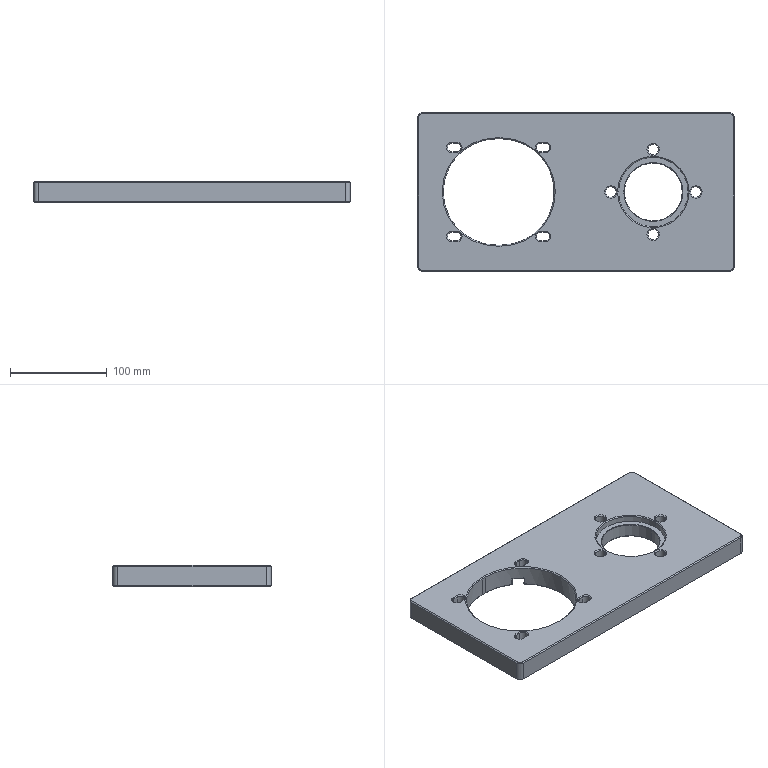NC program | NX | posted with a generic post | part box 328 x 164 x 22 mm
Lines 5257 to 5344 of 34171:
(ZLEVEL_PROFILE_COPY , TOOL : D10JING)
N10470 T09 M6
N10472 G54
N10474 G17 G0 G90 X-156.096 Y-88. S5000 M3
N10476 G43 Z30. H9
N10478 Z-21.
N10480 G94 G1 Z-22. F1000.
N10482 X-156.388 Y-87.496
N10484 G3 X-157.255 Y-86.998 R1.
N10486 G1 X-158.596 Y-87.
N10488 X-159.011
N10490 G2 X-169. Y-77. R10.
N10492 G1 Y-76.596
N10494 X-168.998 Y-75.255
N10496 G3 X-169.496 Y-74.388 R1.
N10498 G1 X-170. Y-74.096
N10500 Z-21.
N10502 G0 Z30.
N10504 Y74.096
N10506 Z-21.
N10508 G1 Z-22.
N10510 X-169.496 Y74.388
N10512 G3 X-168.998 Y75.255 R1.
N10514 G1 X-169. Y76.596
N10516 Y77.
N10518 G2 X-159. Y87. R10.
N10520 G1 X-158.596
N10522 X-157.255
N10524 G3 X-156.389 Y87.5 R1.
N10526 G1 X-156.1 Y88.
N10528 Z-21.
N10530 G0 Z30.
N10532 X156.1
N10534 Z-21.
N10536 G1 Z-22.
N10538 X156.389 Y87.5
N10540 G3 X157.255 Y87. R1.
N10542 G1 X158.596
N10544 X159.
N10546 G2 X169. Y77. R10.
N10548 G1 Y76.596
N10550 Y75.255
N10552 G3 X169.5 Y74.389 R1.
N10554 G1 X170. Y74.1
N10556 Z-21.
N10558 G0 Z30.
N10560 Y-74.1
N10562 Z-21.
N10564 G1 Z-22.
N10566 X169.5 Y-74.389
N10568 G3 X169. Y-75.255 R1.
N10570 G1 Y-76.596
N10572 Y-77.011
N10574 G2 X158.985 Y-87. R10.
N10576 G1 X158.596
N10578 X157.255 Y-86.998
N10580 G3 X156.388 Y-87.496 R1.
N10582 G1 X156.096 Y-88.
N10584 Z-21.
N10586 G0 Z30.
(ZLEVEL_PROFILE_COPY_COPY , TOOL : D10JING)
N10588 X57.973 Y9.529
N10590 Z-21.
N10592 G1 Z-22.
N10594 X57.371 Y9.429
N10596 G3 X56.598 Y8.794 R1.
N10598 X55.406 Y4.486 R25.
N10600 G1 X55.412 Y4.471
N10602 X55.401 Y4.458
N10604 G3 X55.401 Y-4.458 R25.
N10606 G1 X55.412 Y-4.471
N10608 X55.406 Y-4.486
N10610 G3 X104.594 Y-4.486 R25.
N10612 G1 X104.588 Y-4.471
N10614 X104.599 Y-4.458
N10616 G3 X104.599 Y4.458 R25.
N10618 G1 X104.588 Y4.471
N10620 X104.594 Y4.486
N10622 G3 X56.598 Y8.794 R25.
N10624 X56.761 Y7.808 R1.
N10626 G1 X57.149 Y7.336
N10628 Z-21.
N10630 G0 Z30.
N10632 M5